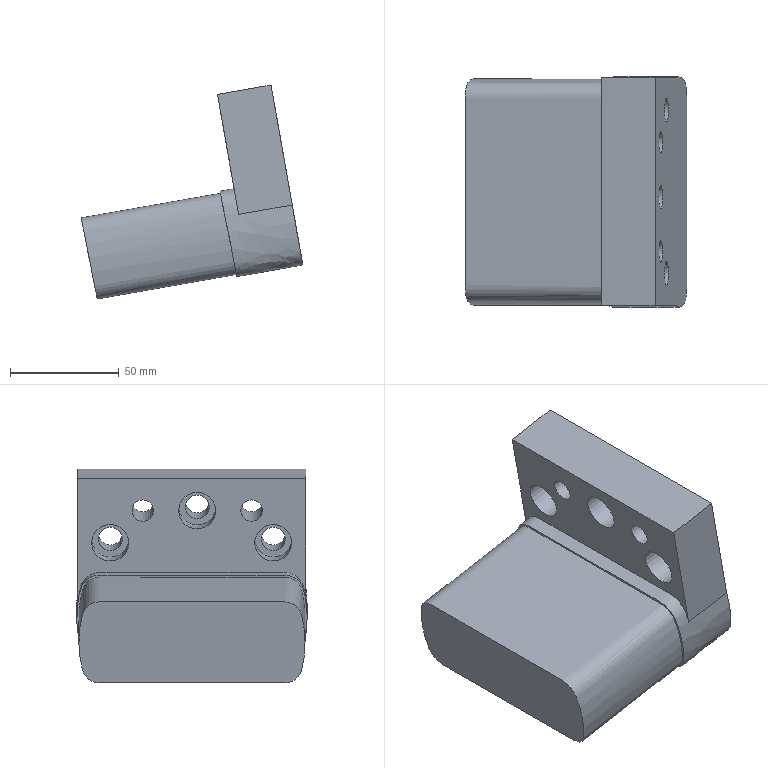Part | NX | features solid 2 | 1 solid | 20 faces | box 101.88 x 105.983 x 98.4 mm | volume 483853 mm3 | plane 8 | cylinder 8 | spline 4 | commonest cylinder face diameters 11 x3 17 x3 10 x2